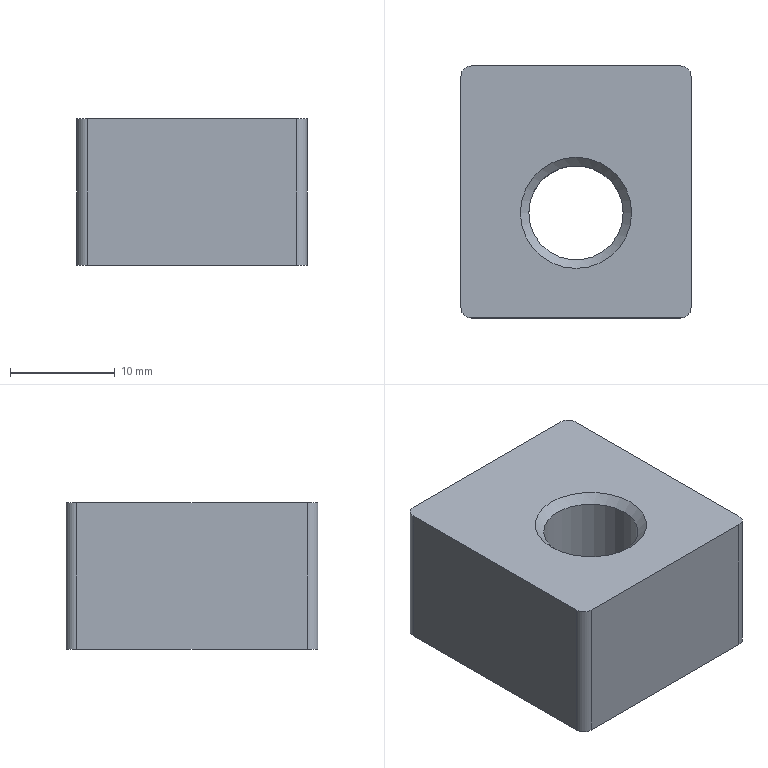Part | NX | 1 solid | 13 faces | box 21.95 x 24 x 14 mm | volume 6453 mm3 | plane 6 | cylinder 5 | cone 2 | commonest cylinder face diameters 2 x4 9 x1
STEP:
#1=CARTESIAN_POINT('',(16.275,10.,20.));
#2=VERTEX_POINT('',#1);
#3=CARTESIAN_POINT('',(10.975,10.,20.));
#4=DIRECTION('',(0.,0.,1.));
#5=DIRECTION('',(1.,0.,0.));
#6=AXIS2_PLACEMENT_3D('',#3,#4,#5);
#7=CIRCLE('',#6,5.3);
#8=EDGE_CURVE('',#2,#2,#7,.F.);
#9=ORIENTED_EDGE('',*,*,#8,.T.);
#10=EDGE_LOOP('',(#9));
#11=FACE_BOUND('',#10,.T.);
#12=CARTESIAN_POINT('',(0.,1.,20.));
#13=VERTEX_POINT('',#12);
#14=CARTESIAN_POINT('',(0.,23.,20.));
#15=VERTEX_POINT('',#14);
#16=CARTESIAN_POINT('',(0.,12.,20.));
#17=DIRECTION('',(0.,1.,0.));
#18=VECTOR('',#17,1000.);
#19=LINE('',#16,#18);
#20=EDGE_CURVE('',#13,#15,#19,.T.);
#21=ORIENTED_EDGE('',*,*,#20,.F.);
#22=CARTESIAN_POINT('',(1.,0.,20.));
#23=VERTEX_POINT('',#22);
#24=CARTESIAN_POINT('',(1.,1.,20.));
#25=DIRECTION('',(0.,0.,1.));
#26=DIRECTION('',(1.,0.,0.));
#27=AXIS2_PLACEMENT_3D('',#24,#25,#26);
#28=CIRCLE('',#27,1.);
#29=EDGE_CURVE('',#13,#23,#28,.T.);
#30=ORIENTED_EDGE('',*,*,#29,.T.);
#31=CARTESIAN_POINT('',(20.95,0.,20.));
#32=VERTEX_POINT('',#31);
#33=CARTESIAN_POINT('',(10.975,0.,20.));
#34=DIRECTION('',(-1.,0.,0.));
#35=VECTOR('',#34,1000.);
#36=LINE('',#33,#35);
#37=EDGE_CURVE('',#32,#23,#36,.T.);
#38=ORIENTED_EDGE('',*,*,#37,.F.);
#39=CARTESIAN_POINT('',(21.95,1.,20.));
#40=VERTEX_POINT('',#39);
#41=CARTESIAN_POINT('',(20.95,1.,20.));
#42=DIRECTION('',(0.,0.,1.));
#43=DIRECTION('',(1.,0.,0.));
#44=AXIS2_PLACEMENT_3D('',#41,#42,#43);
#45=CIRCLE('',#44,1.);
#46=EDGE_CURVE('',#32,#40,#45,.T.);
#47=ORIENTED_EDGE('',*,*,#46,.T.);
#48=CARTESIAN_POINT('',(21.95,23.,20.));
#49=VERTEX_POINT('',#48);
#50=CARTESIAN_POINT('',(21.95,12.,20.));
#51=DIRECTION('',(0.,-1.,0.));
#52=VECTOR('',#51,1000.);
#53=LINE('',#50,#52);
#54=EDGE_CURVE('',#49,#40,#53,.T.);
#55=ORIENTED_EDGE('',*,*,#54,.F.);
#56=CARTESIAN_POINT('',(20.95,24.,20.));
#57=VERTEX_POINT('',#56);
#58=CARTESIAN_POINT('',(20.95,23.,20.));
#59=DIRECTION('',(0.,0.,1.));
#60=DIRECTION('',(1.,0.,0.));
#61=AXIS2_PLACEMENT_3D('',#58,#59,#60);
#62=CIRCLE('',#61,1.);
#63=EDGE_CURVE('',#49,#57,#62,.T.);
#64=ORIENTED_EDGE('',*,*,#63,.T.);
#65=CARTESIAN_POINT('',(1.,24.,20.));
#66=VERTEX_POINT('',#65);
#67=CARTESIAN_POINT('',(10.975,24.,20.));
#68=DIRECTION('',(1.,0.,0.));
#69=VECTOR('',#68,1000.);
#70=LINE('',#67,#69);
#71=EDGE_CURVE('',#66,#57,#70,.T.);
#72=ORIENTED_EDGE('',*,*,#71,.F.);
#73=CARTESIAN_POINT('',(1.,23.,20.));
#74=DIRECTION('',(0.,0.,1.));
#75=DIRECTION('',(1.,0.,0.));
#76=AXIS2_PLACEMENT_3D('',#73,#74,#75);
#77=CIRCLE('',#76,1.);
#78=EDGE_CURVE('',#66,#15,#77,.T.);
#79=ORIENTED_EDGE('',*,*,#78,.T.);
#80=EDGE_LOOP('',(#21,#30,#38,#47,#55,#64,#72,#79));
#81=FACE_BOUND('',#80,.T.);
#82=CARTESIAN_POINT('',(10.975,12.,20.));
#83=DIRECTION('',(0.,0.,1.));
#84=DIRECTION('',(1.,0.,0.));
#85=AXIS2_PLACEMENT_3D('',#82,#83,#84);
#86=PLANE('',#85);
#87=ADVANCED_FACE('',(#11,#81),#86,.T.);
#88=ORIENTED_EDGE('',*,*,#37,.T.);
#89=CARTESIAN_POINT('',(1.,0.,6.));
#90=VERTEX_POINT('',#89);
#91=CARTESIAN_POINT('',(1.,0.,0.));
#92=DIRECTION('',(0.,0.,1.));
#93=VECTOR('',#92,1000.);
#94=LINE('',#91,#93);
#95=EDGE_CURVE('',#23,#90,#94,.F.);
#96=ORIENTED_EDGE('',*,*,#95,.T.);
#97=CARTESIAN_POINT('',(20.95,0.,6.));
#98=VERTEX_POINT('',#97);
#99=CARTESIAN_POINT('',(10.975,0.,6.));
#100=DIRECTION('',(1.,0.,0.));
#101=VECTOR('',#100,1000.);
#102=LINE('',#99,#101);
#103=EDGE_CURVE('',#90,#98,#102,.T.);
#104=ORIENTED_EDGE('',*,*,#103,.T.);
#105=CARTESIAN_POINT('',(20.95,0.,0.));
#106=DIRECTION('',(0.,0.,1.));
#107=VECTOR('',#106,1000.);
#108=LINE('',#105,#107);
#109=EDGE_CURVE('',#98,#32,#108,.T.);
#110=ORIENTED_EDGE('',*,*,#109,.T.);
#111=EDGE_LOOP('',(#88,#96,#104,#110));
#112=FACE_BOUND('',#111,.T.);
#113=CARTESIAN_POINT('',(10.975,0.,0.));
#114=DIRECTION('',(0.,-1.,0.));
#115=DIRECTION('',(0.,0.,-1.));
#116=AXIS2_PLACEMENT_3D('',#113,#114,#115);
#117=PLANE('',#116);
#118=ADVANCED_FACE('',(#112),#117,.T.);
#119=CARTESIAN_POINT('',(0.,23.,6.));
#120=VERTEX_POINT('',#119);
#121=CARTESIAN_POINT('',(0.,1.,6.));
#122=VERTEX_POINT('',#121);
#123=CARTESIAN_POINT('',(0.,12.,6.));
#124=DIRECTION('',(0.,-1.,0.));
#125=VECTOR('',#124,1000.);
#126=LINE('',#123,#125);
#127=EDGE_CURVE('',#120,#122,#126,.T.);
#128=ORIENTED_EDGE('',*,*,#127,.T.);
#129=CARTESIAN_POINT('',(0.,1.,0.));
#130=DIRECTION('',(0.,0.,1.));
#131=VECTOR('',#130,1000.);
#132=LINE('',#129,#131);
#133=EDGE_CURVE('',#122,#13,#132,.T.);
#134=ORIENTED_EDGE('',*,*,#133,.T.);
#135=ORIENTED_EDGE('',*,*,#20,.T.);
#136=CARTESIAN_POINT('',(0.,23.,0.));
#137=DIRECTION('',(0.,0.,1.));
#138=VECTOR('',#137,1000.);
#139=LINE('',#136,#138);
#140=EDGE_CURVE('',#15,#120,#139,.F.);
#141=ORIENTED_EDGE('',*,*,#140,.T.);
#142=EDGE_LOOP('',(#128,#134,#135,#141));
#143=FACE_BOUND('',#142,.T.);
#144=CARTESIAN_POINT('',(0.,12.,0.));
#145=DIRECTION('',(-1.,0.,0.));
#146=DIRECTION('',(0.,0.,1.));
#147=AXIS2_PLACEMENT_3D('',#144,#145,#146);
#148=PLANE('',#147);
#149=ADVANCED_FACE('',(#143),#148,.T.);
#150=CARTESIAN_POINT('',(20.95,24.,6.));
#151=VERTEX_POINT('',#150);
#152=CARTESIAN_POINT('',(1.,24.,6.));
#153=VERTEX_POINT('',#152);
#154=CARTESIAN_POINT('',(10.975,24.,6.));
#155=DIRECTION('',(-1.,0.,0.));
#156=VECTOR('',#155,1000.);
#157=LINE('',#154,#156);
#158=EDGE_CURVE('',#151,#153,#157,.T.);
#159=ORIENTED_EDGE('',*,*,#158,.T.);
#160=CARTESIAN_POINT('',(1.,24.,0.));
#161=DIRECTION('',(0.,0.,1.));
#162=VECTOR('',#161,1000.);
#163=LINE('',#160,#162);
#164=EDGE_CURVE('',#153,#66,#163,.T.);
#165=ORIENTED_EDGE('',*,*,#164,.T.);
#166=ORIENTED_EDGE('',*,*,#71,.T.);
#167=CARTESIAN_POINT('',(20.95,24.,0.));
#168=DIRECTION('',(0.,0.,1.));
#169=VECTOR('',#168,1000.);
#170=LINE('',#167,#169);
#171=EDGE_CURVE('',#57,#151,#170,.F.);
#172=ORIENTED_EDGE('',*,*,#171,.T.);
#173=EDGE_LOOP('',(#159,#165,#166,#172));
#174=FACE_BOUND('',#173,.T.);
#175=CARTESIAN_POINT('',(10.975,24.,0.));
#176=DIRECTION('',(0.,1.,0.));
#177=DIRECTION('',(0.,0.,1.));
#178=AXIS2_PLACEMENT_3D('',#175,#176,#177);
#179=PLANE('',#178);
#180=ADVANCED_FACE('',(#174),#179,.T.);
#181=CARTESIAN_POINT('',(5.675,10.,6.));
#182=VERTEX_POINT('',#181);
#183=CARTESIAN_POINT('',(10.975,10.,6.));
#184=DIRECTION('',(0.,0.,-1.));
#185=DIRECTION('',(-1.,0.,0.));
#186=AXIS2_PLACEMENT_3D('',#183,#184,#185);
#187=CIRCLE('',#186,5.3);
#188=EDGE_CURVE('',#182,#182,#187,.F.);
#189=ORIENTED_EDGE('',*,*,#188,.T.);
#190=EDGE_LOOP('',(#189));
#191=FACE_BOUND('',#190,.T.);
#192=ORIENTED_EDGE('',*,*,#103,.F.);
#193=CARTESIAN_POINT('',(1.,1.,6.));
#194=DIRECTION('',(0.,0.,-1.));
#195=DIRECTION('',(-1.,0.,0.));
#196=AXIS2_PLACEMENT_3D('',#193,#194,#195);
#197=CIRCLE('',#196,1.);
#198=EDGE_CURVE('',#90,#122,#197,.T.);
#199=ORIENTED_EDGE('',*,*,#198,.T.);
#200=ORIENTED_EDGE('',*,*,#127,.F.);
#201=CARTESIAN_POINT('',(1.,23.,6.));
#202=DIRECTION('',(0.,0.,-1.));
#203=DIRECTION('',(-1.,0.,0.));
#204=AXIS2_PLACEMENT_3D('',#201,#202,#203);
#205=CIRCLE('',#204,1.);
#206=EDGE_CURVE('',#120,#153,#205,.T.);
#207=ORIENTED_EDGE('',*,*,#206,.T.);
#208=ORIENTED_EDGE('',*,*,#158,.F.);
#209=CARTESIAN_POINT('',(21.95,23.,6.));
#210=VERTEX_POINT('',#209);
#211=CARTESIAN_POINT('',(20.95,23.,6.));
#212=DIRECTION('',(0.,0.,-1.));
#213=DIRECTION('',(-1.,0.,0.));
#214=AXIS2_PLACEMENT_3D('',#211,#212,#213);
#215=CIRCLE('',#214,1.);
#216=EDGE_CURVE('',#151,#210,#215,.T.);
#217=ORIENTED_EDGE('',*,*,#216,.T.);
#218=CARTESIAN_POINT('',(21.95,1.,6.));
#219=VERTEX_POINT('',#218);
#220=CARTESIAN_POINT('',(21.95,12.,6.));
#221=DIRECTION('',(0.,1.,0.));
#222=VECTOR('',#221,1000.);
#223=LINE('',#220,#222);
#224=EDGE_CURVE('',#219,#210,#223,.T.);
#225=ORIENTED_EDGE('',*,*,#224,.F.);
#226=CARTESIAN_POINT('',(20.95,1.,6.));
#227=DIRECTION('',(0.,0.,-1.));
#228=DIRECTION('',(-1.,0.,0.));
#229=AXIS2_PLACEMENT_3D('',#226,#227,#228);
#230=CIRCLE('',#229,1.);
#231=EDGE_CURVE('',#219,#98,#230,.T.);
#232=ORIENTED_EDGE('',*,*,#231,.T.);
#233=EDGE_LOOP('',(#192,#199,#200,#207,#208,#217,#225,#232));
#234=FACE_BOUND('',#233,.T.);
#235=CARTESIAN_POINT('',(10.975,12.,6.));
#236=DIRECTION('',(0.,0.,-1.));
#237=DIRECTION('',(-1.,0.,0.));
#238=AXIS2_PLACEMENT_3D('',#235,#236,#237);
#239=PLANE('',#238);
#240=ADVANCED_FACE('',(#191,#234),#239,.T.);
#241=ORIENTED_EDGE('',*,*,#224,.T.);
#242=CARTESIAN_POINT('',(21.95,23.,0.));
#243=DIRECTION('',(0.,0.,1.));
#244=VECTOR('',#243,1000.);
#245=LINE('',#242,#244);
#246=EDGE_CURVE('',#210,#49,#245,.T.);
#247=ORIENTED_EDGE('',*,*,#246,.T.);
#248=ORIENTED_EDGE('',*,*,#54,.T.);
#249=CARTESIAN_POINT('',(21.95,1.,0.));
#250=DIRECTION('',(0.,0.,1.));
#251=VECTOR('',#250,1000.);
#252=LINE('',#249,#251);
#253=EDGE_CURVE('',#40,#219,#252,.F.);
#254=ORIENTED_EDGE('',*,*,#253,.T.);
#255=EDGE_LOOP('',(#241,#247,#248,#254));
#256=FACE_BOUND('',#255,.T.);
#257=CARTESIAN_POINT('',(21.95,12.,0.));
#258=DIRECTION('',(1.,0.,0.));
#259=DIRECTION('',(0.,0.,-1.));
#260=AXIS2_PLACEMENT_3D('',#257,#258,#259);
#261=PLANE('',#260);
#262=ADVANCED_FACE('',(#256),#261,.T.);
#263=CARTESIAN_POINT('',(6.475,10.,6.8));
#264=VERTEX_POINT('',#263);
#265=CARTESIAN_POINT('',(10.975,10.,6.8));
#266=DIRECTION('',(0.,0.,-1.));
#267=DIRECTION('',(-1.,0.,0.));
#268=AXIS2_PLACEMENT_3D('',#265,#266,#267);
#269=CIRCLE('',#268,4.5);
#270=EDGE_CURVE('',#264,#264,#269,.T.);
#271=ORIENTED_EDGE('',*,*,#270,.T.);
#272=EDGE_LOOP('',(#271));
#273=FACE_BOUND('',#272,.T.);
#274=CARTESIAN_POINT('',(15.475,10.,19.2));
#275=VERTEX_POINT('',#274);
#276=CARTESIAN_POINT('',(10.975,10.,19.2));
#277=DIRECTION('',(0.,0.,1.));
#278=DIRECTION('',(1.,0.,0.));
#279=AXIS2_PLACEMENT_3D('',#276,#277,#278);
#280=CIRCLE('',#279,4.5);
#281=EDGE_CURVE('',#275,#275,#280,.T.);
#282=ORIENTED_EDGE('',*,*,#281,.T.);
#283=EDGE_LOOP('',(#282));
#284=FACE_BOUND('',#283,.T.);
#285=CARTESIAN_POINT('',(10.975,10.,20.));
#286=DIRECTION('',(0.,0.,-1.));
#287=DIRECTION('',(-1.,0.,0.));
#288=AXIS2_PLACEMENT_3D('',#285,#286,#287);
#289=CYLINDRICAL_SURFACE('',#288,4.5);
#290=ADVANCED_FACE('',(#273,#284),#289,.F.);
#291=ORIENTED_EDGE('',*,*,#198,.F.);
#292=ORIENTED_EDGE('',*,*,#95,.F.);
#293=ORIENTED_EDGE('',*,*,#29,.F.);
#294=ORIENTED_EDGE('',*,*,#133,.F.);
#295=EDGE_LOOP('',(#291,#292,#293,#294));
#296=FACE_BOUND('',#295,.T.);
#297=CARTESIAN_POINT('',(1.,1.,0.));
#298=DIRECTION('',(0.,0.,1.));
#299=DIRECTION('',(1.,0.,0.));
#300=AXIS2_PLACEMENT_3D('',#297,#298,#299);
#301=CYLINDRICAL_SURFACE('',#300,1.);
#302=ADVANCED_FACE('',(#296),#301,.T.);
#303=ORIENTED_EDGE('',*,*,#206,.F.);
#304=ORIENTED_EDGE('',*,*,#140,.F.);
#305=ORIENTED_EDGE('',*,*,#78,.F.);
#306=ORIENTED_EDGE('',*,*,#164,.F.);
#307=EDGE_LOOP('',(#303,#304,#305,#306));
#308=FACE_BOUND('',#307,.T.);
#309=CARTESIAN_POINT('',(1.,23.,0.));
#310=DIRECTION('',(0.,0.,1.));
#311=DIRECTION('',(1.,0.,0.));
#312=AXIS2_PLACEMENT_3D('',#309,#310,#311);
#313=CYLINDRICAL_SURFACE('',#312,1.);
#314=ADVANCED_FACE('',(#308),#313,.T.);
#315=ORIENTED_EDGE('',*,*,#216,.F.);
#316=ORIENTED_EDGE('',*,*,#171,.F.);
#317=ORIENTED_EDGE('',*,*,#63,.F.);
#318=ORIENTED_EDGE('',*,*,#246,.F.);
#319=EDGE_LOOP('',(#315,#316,#317,#318));
#320=FACE_BOUND('',#319,.T.);
#321=CARTESIAN_POINT('',(20.95,23.,0.));
#322=DIRECTION('',(0.,0.,1.));
#323=DIRECTION('',(1.,0.,0.));
#324=AXIS2_PLACEMENT_3D('',#321,#322,#323);
#325=CYLINDRICAL_SURFACE('',#324,1.);
#326=ADVANCED_FACE('',(#320),#325,.T.);
#327=ORIENTED_EDGE('',*,*,#231,.F.);
#328=ORIENTED_EDGE('',*,*,#253,.F.);
#329=ORIENTED_EDGE('',*,*,#46,.F.);
#330=ORIENTED_EDGE('',*,*,#109,.F.);
#331=EDGE_LOOP('',(#327,#328,#329,#330));
#332=FACE_BOUND('',#331,.T.);
#333=CARTESIAN_POINT('',(20.95,1.,0.));
#334=DIRECTION('',(0.,0.,1.));
#335=DIRECTION('',(1.,0.,0.));
#336=AXIS2_PLACEMENT_3D('',#333,#334,#335);
#337=CYLINDRICAL_SURFACE('',#336,1.);
#338=ADVANCED_FACE('',(#332),#337,.T.);
#339=ORIENTED_EDGE('',*,*,#188,.F.);
#340=EDGE_LOOP('',(#339));
#341=FACE_BOUND('',#340,.T.);
#342=ORIENTED_EDGE('',*,*,#270,.F.);
#343=EDGE_LOOP('',(#342));
#344=FACE_BOUND('',#343,.T.);
#345=CARTESIAN_POINT('',(10.975,10.,6.8));
#346=DIRECTION('',(0.,0.,-1.));
#347=DIRECTION('',(-1.,0.,0.));
#348=AXIS2_PLACEMENT_3D('',#345,#346,#347);
#349=CONICAL_SURFACE('',#348,4.5,0.7854);
#350=ADVANCED_FACE('',(#341,#344),#349,.F.);
#351=ORIENTED_EDGE('',*,*,#281,.F.);
#352=EDGE_LOOP('',(#351));
#353=FACE_BOUND('',#352,.T.);
#354=ORIENTED_EDGE('',*,*,#8,.F.);
#355=EDGE_LOOP('',(#354));
#356=FACE_BOUND('',#355,.T.);
#357=CARTESIAN_POINT('',(10.975,10.,20.));
#358=DIRECTION('',(0.,0.,1.));
#359=DIRECTION('',(1.,0.,0.));
#360=AXIS2_PLACEMENT_3D('',#357,#358,#359);
#361=CONICAL_SURFACE('',#360,5.3,0.7854);
#362=ADVANCED_FACE('',(#353,#356),#361,.F.);
#363=CLOSED_SHELL('',(#87,#118,#149,#180,#240,#262,#290,#302,#314,#326,#338,#350,#362));
#364=MANIFOLD_SOLID_BREP('',#363);
#365=(LENGTH_UNIT()NAMED_UNIT(*)SI_UNIT(.MILLI.,.METRE.));
#366=UNCERTAINTY_MEASURE_WITH_UNIT(LENGTH_MEASURE(0.00001),#365,'','');
#367=(NAMED_UNIT(*)PLANE_ANGLE_UNIT()SI_UNIT($,.RADIAN.));
#368=(NAMED_UNIT(*)SI_UNIT($,.STERADIAN.)SOLID_ANGLE_UNIT());
#369=(GEOMETRIC_REPRESENTATION_CONTEXT(3)GLOBAL_UNCERTAINTY_ASSIGNED_CONTEXT((#366))GLOBAL_UNIT_ASSIGNED_CONTEXT((#365,#367,#368))REPRESENTATION_CONTEXT('',''));
#370=ADVANCED_BREP_SHAPE_REPRESENTATION('',(#364),#369);